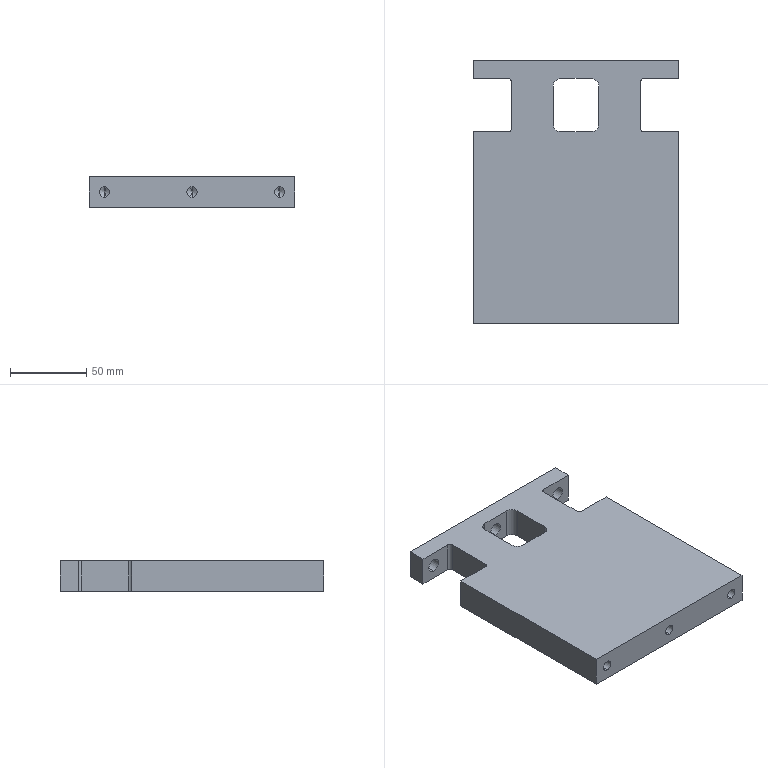Part | STEP file | 0229_202_Plate | 1 solid | 44 faces | box 135 x 173 x 20 mm | volume 406809 mm3 | cylinder 20 | plane 18 | cone 6 | commonest cylinder face diameters 6.8 x6 9 x6 4 x4 10 x4